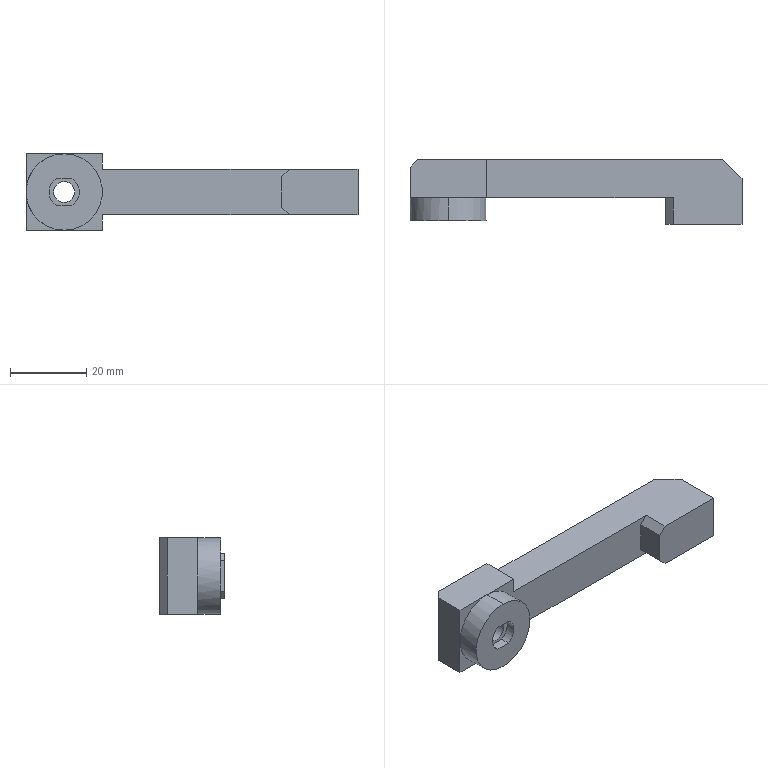Part | STEP file | ASND-0110-clamp 12 | 1 solid | 31 faces | box 87 x 17 x 20 mm | volume 14618 mm3 | plane 23 | cylinder 8 | commonest cylinder face diameters 5.5 x2 8 x2 10 x2 20 x2